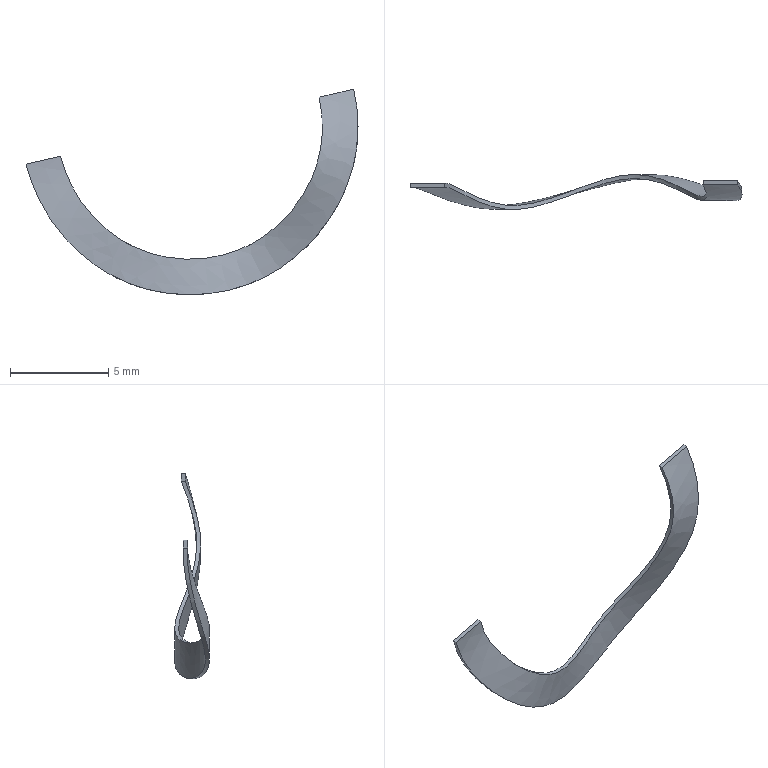Part | NX | features ODD_TURNS_COMBINE 2 | 1 solid | 6 faces | box 16.858 x 1.775 x 10.436 mm | volume 8.764 mm3 | spline 4 | plane 2
STEP:
#1=CARTESIAN_POINT('',(-8.32,-24.173,-1.899));
#2=VERTEX_POINT('',#1);
#3=CARTESIAN_POINT('',(-8.32,-23.97,-1.899));
#4=VERTEX_POINT('',#3);
#5=CARTESIAN_POINT('',(-8.32,-23.97,-1.899));
#6=CARTESIAN_POINT('',(-8.32,-24.037,-1.899));
#7=CARTESIAN_POINT('',(-8.32,-24.105,-1.899));
#8=CARTESIAN_POINT('',(-8.32,-24.173,-1.899));
#9=B_SPLINE_CURVE_WITH_KNOTS('',3,(#5,#6,#7,#8),.UNSPECIFIED.,.F.,.F.,(4,4),(0.,0.0002032),.UNSPECIFIED.);
#10=EDGE_CURVE('',#2,#4,#9,.F.);
#11=ORIENTED_EDGE('',*,*,#10,.T.);
#12=CARTESIAN_POINT('',(8.322,-23.865,1.899));
#13=VERTEX_POINT('',#12);
#14=CARTESIAN_POINT('',(-3.703,-25.301,-7.689));
#15=CARTESIAN_POINT('',(-1.417,-25.248,-8.753));
#16=CARTESIAN_POINT('',(4.289,-27.759,-8.773));
#17=CARTESIAN_POINT('',(9.501,-23.516,-2.229));
#18=CARTESIAN_POINT('',(7.592,-27.322,6.131));
#19=CARTESIAN_POINT('',(0.06027,-23.071,9.76));
#20=CARTESIAN_POINT('',(-7.667,-26.878,6.037));
#21=CARTESIAN_POINT('',(-9.528,-22.627,-2.113));
#22=CARTESIAN_POINT('',(-4.18,-26.435,-8.819));
#23=CARTESIAN_POINT('',(4.18,-22.183,-8.819));
#24=CARTESIAN_POINT('',(9.527,-25.991,-2.113));
#25=CARTESIAN_POINT('',(7.668,-21.74,6.038));
#26=CARTESIAN_POINT('',(-0.06063,-25.547,9.759));
#27=CARTESIAN_POINT('',(-7.591,-21.298,6.133));
#28=CARTESIAN_POINT('',(-8.865,-23.825,0.5668));
#29=CARTESIAN_POINT('',(-8.32,-23.761,-1.899));
#30=B_SPLINE_CURVE_WITH_KNOTS('',3,(#14,#15,#16,#17,#18,#19,#20,#21,#22,#23,#24,#25,#26,#27,#28,#29),.UNSPECIFIED.,.F.,.F.,(4,1,1,1,1,1,1,1,1,1,1,1,1,4),(0.,0.07646,0.1539,0.2304,0.3078,0.3843,0.4618,0.5382,0.6157,0.6922,0.7696,0.8461,0.9235,1.),.UNSPECIFIED.);
#31=EDGE_CURVE('',#4,#13,#30,.T.);
#32=ORIENTED_EDGE('',*,*,#31,.T.);
#33=CARTESIAN_POINT('',(8.322,-24.069,1.899));
#34=VERTEX_POINT('',#33);
#35=CARTESIAN_POINT('',(8.322,-24.069,1.899));
#36=CARTESIAN_POINT('',(8.322,-24.001,1.899));
#37=CARTESIAN_POINT('',(8.322,-23.933,1.899));
#38=CARTESIAN_POINT('',(8.322,-23.865,1.899));
#39=B_SPLINE_CURVE_WITH_KNOTS('',3,(#35,#36,#37,#38),.UNSPECIFIED.,.F.,.F.,(4,4),(0.,0.0002032),.UNSPECIFIED.);
#40=EDGE_CURVE('',#13,#34,#39,.F.);
#41=ORIENTED_EDGE('',*,*,#40,.T.);
#42=CARTESIAN_POINT('',(-3.703,-25.504,-7.689));
#43=CARTESIAN_POINT('',(-1.417,-25.451,-8.753));
#44=CARTESIAN_POINT('',(4.289,-27.962,-8.773));
#45=CARTESIAN_POINT('',(9.501,-23.72,-2.229));
#46=CARTESIAN_POINT('',(7.592,-27.525,6.131));
#47=CARTESIAN_POINT('',(0.06027,-23.274,9.76));
#48=CARTESIAN_POINT('',(-7.667,-27.082,6.037));
#49=CARTESIAN_POINT('',(-9.528,-22.83,-2.113));
#50=CARTESIAN_POINT('',(-4.18,-26.638,-8.819));
#51=CARTESIAN_POINT('',(4.18,-22.387,-8.819));
#52=CARTESIAN_POINT('',(9.527,-26.194,-2.113));
#53=CARTESIAN_POINT('',(7.668,-21.943,6.038));
#54=CARTESIAN_POINT('',(-0.06063,-25.75,9.759));
#55=CARTESIAN_POINT('',(-7.591,-21.501,6.133));
#56=CARTESIAN_POINT('',(-8.865,-24.028,0.5668));
#57=CARTESIAN_POINT('',(-8.32,-23.964,-1.899));
#58=B_SPLINE_CURVE_WITH_KNOTS('',3,(#42,#43,#44,#45,#46,#47,#48,#49,#50,#51,#52,#53,#54,#55,#56,#57),.UNSPECIFIED.,.F.,.F.,(4,1,1,1,1,1,1,1,1,1,1,1,1,4),(0.,0.07646,0.1539,0.2304,0.3078,0.3843,0.4618,0.5382,0.6157,0.6922,0.7696,0.8461,0.9235,1.),.UNSPECIFIED.);
#59=EDGE_CURVE('',#2,#34,#58,.T.);
#60=ORIENTED_EDGE('',*,*,#59,.F.);
#61=EDGE_LOOP('',(#11,#32,#41,#60));
#62=FACE_BOUND('',#61,.T.);
#63=CARTESIAN_POINT('',(-8.32,-24.173,-1.899));
#64=CARTESIAN_POINT('',(-7.737,-24.105,-4.358));
#65=CARTESIAN_POINT('',(-4.18,-26.638,-8.819));
#66=CARTESIAN_POINT('',(4.18,-22.387,-8.819));
#67=CARTESIAN_POINT('',(8.632,-25.557,-3.235));
#68=CARTESIAN_POINT('',(8.606,-24.443,0.6545));
#69=CARTESIAN_POINT('',(8.322,-24.069,1.899));
#70=CARTESIAN_POINT('',(-8.32,-24.156,-1.899));
#71=CARTESIAN_POINT('',(-7.737,-24.088,-4.358));
#72=CARTESIAN_POINT('',(-4.18,-26.621,-8.819));
#73=CARTESIAN_POINT('',(4.18,-22.37,-8.819));
#74=CARTESIAN_POINT('',(8.632,-25.54,-3.235));
#75=CARTESIAN_POINT('',(8.606,-24.426,0.6545));
#76=CARTESIAN_POINT('',(8.322,-24.052,1.899));
#77=CARTESIAN_POINT('',(-8.32,-24.122,-1.899));
#78=CARTESIAN_POINT('',(-7.737,-24.054,-4.358));
#79=CARTESIAN_POINT('',(-4.18,-26.587,-8.819));
#80=CARTESIAN_POINT('',(4.18,-22.336,-8.819));
#81=CARTESIAN_POINT('',(8.632,-25.506,-3.235));
#82=CARTESIAN_POINT('',(8.606,-24.392,0.6545));
#83=CARTESIAN_POINT('',(8.322,-24.018,1.899));
#84=CARTESIAN_POINT('',(-8.32,-24.071,-1.899));
#85=CARTESIAN_POINT('',(-7.737,-24.003,-4.358));
#86=CARTESIAN_POINT('',(-4.18,-26.536,-8.819));
#87=CARTESIAN_POINT('',(4.18,-22.285,-8.819));
#88=CARTESIAN_POINT('',(8.632,-25.455,-3.235));
#89=CARTESIAN_POINT('',(8.606,-24.342,0.6545));
#90=CARTESIAN_POINT('',(8.322,-23.967,1.899));
#91=CARTESIAN_POINT('',(-8.32,-24.02,-1.899));
#92=CARTESIAN_POINT('',(-7.737,-23.953,-4.358));
#93=CARTESIAN_POINT('',(-4.18,-26.486,-8.819));
#94=CARTESIAN_POINT('',(4.18,-22.234,-8.819));
#95=CARTESIAN_POINT('',(8.632,-25.404,-3.235));
#96=CARTESIAN_POINT('',(8.606,-24.291,0.6545));
#97=CARTESIAN_POINT('',(8.322,-23.916,1.899));
#98=CARTESIAN_POINT('',(-8.32,-23.986,-1.899));
#99=CARTESIAN_POINT('',(-7.737,-23.919,-4.358));
#100=CARTESIAN_POINT('',(-4.18,-26.452,-8.819));
#101=CARTESIAN_POINT('',(4.18,-22.2,-8.819));
#102=CARTESIAN_POINT('',(8.632,-25.371,-3.235));
#103=CARTESIAN_POINT('',(8.606,-24.257,0.6545));
#104=CARTESIAN_POINT('',(8.322,-23.882,1.899));
#105=CARTESIAN_POINT('',(-8.32,-23.97,-1.899));
#106=CARTESIAN_POINT('',(-7.737,-23.902,-4.358));
#107=CARTESIAN_POINT('',(-4.18,-26.435,-8.819));
#108=CARTESIAN_POINT('',(4.18,-22.183,-8.819));
#109=CARTESIAN_POINT('',(8.632,-25.354,-3.235));
#110=CARTESIAN_POINT('',(8.606,-24.24,0.6545));
#111=CARTESIAN_POINT('',(8.322,-23.865,1.899));
#112=B_SPLINE_SURFACE_WITH_KNOTS('',3,3,((#63,#64,#65,#66,#67,#68,#69),(#70,#71,#72,#73,#74,#75,#76),(#77,#78,#79,#80,#81,#82,#83),(#84,#85,#86,#87,#88,#89,#90),(#91,#92,#93,#94,#95,#96,#97),(#98,#99,#100,#101,#102,#103,#104),(#105,#106,#107,#108,#109,#110,#111)),.SURF_OF_LINEAR_EXTRUSION.,.F.,.F.,.F.,(4,1,1,1,4),(4,1,1,1,4),(0.,0.25,0.5,0.75,1.),(0.4503,0.5,0.5503,0.6,0.6252),.UNSPECIFIED.);
#113=ADVANCED_FACE('',(#62),#112,.T.);
#114=CARTESIAN_POINT('',(-6.562,-24.173,-1.498));
#115=VERTEX_POINT('',#114);
#116=CARTESIAN_POINT('',(-8.32,-24.173,-1.899));
#117=CARTESIAN_POINT('',(-7.734,-24.173,-1.765));
#118=CARTESIAN_POINT('',(-7.148,-24.173,-1.631));
#119=CARTESIAN_POINT('',(-6.562,-24.173,-1.498));
#120=B_SPLINE_CURVE_WITH_KNOTS('',3,(#116,#117,#118,#119),.UNSPECIFIED.,.F.,.F.,(4,4),(0.,0.001803),.UNSPECIFIED.);
#121=EDGE_CURVE('',#2,#115,#120,.T.);
#122=ORIENTED_EDGE('',*,*,#121,.F.);
#123=ORIENTED_EDGE('',*,*,#59,.T.);
#124=CARTESIAN_POINT('',(6.564,-24.069,1.498));
#125=VERTEX_POINT('',#124);
#126=CARTESIAN_POINT('',(6.564,-24.069,1.498));
#127=CARTESIAN_POINT('',(7.15,-24.069,1.632));
#128=CARTESIAN_POINT('',(7.736,-24.069,1.766));
#129=CARTESIAN_POINT('',(8.322,-24.069,1.899));
#130=B_SPLINE_CURVE_WITH_KNOTS('',3,(#126,#127,#128,#129),.UNSPECIFIED.,.F.,.F.,(4,4),(0.,0.001804),.UNSPECIFIED.);
#131=EDGE_CURVE('',#125,#34,#130,.T.);
#132=ORIENTED_EDGE('',*,*,#131,.F.);
#133=CARTESIAN_POINT('',(-2.92,-25.504,-6.064));
#134=CARTESIAN_POINT('',(-1.118,-25.451,-6.904));
#135=CARTESIAN_POINT('',(3.383,-27.962,-6.919));
#136=CARTESIAN_POINT('',(7.493,-23.72,-1.758));
#137=CARTESIAN_POINT('',(5.988,-27.525,4.836));
#138=CARTESIAN_POINT('',(0.04752,-23.274,7.697));
#139=CARTESIAN_POINT('',(-6.047,-27.082,4.761));
#140=CARTESIAN_POINT('',(-7.514,-22.83,-1.666));
#141=CARTESIAN_POINT('',(-3.297,-26.638,-6.955));
#142=CARTESIAN_POINT('',(3.297,-22.387,-6.955));
#143=CARTESIAN_POINT('',(7.514,-26.194,-1.666));
#144=CARTESIAN_POINT('',(6.047,-21.943,4.762));
#145=CARTESIAN_POINT('',(-0.04783,-25.75,7.697));
#146=CARTESIAN_POINT('',(-5.987,-21.501,4.837));
#147=CARTESIAN_POINT('',(-6.991,-24.028,0.447));
#148=CARTESIAN_POINT('',(-6.562,-23.964,-1.498));
#149=B_SPLINE_CURVE_WITH_KNOTS('',3,(#133,#134,#135,#136,#137,#138,#139,#140,#141,#142,#143,#144,#145,#146,#147,#148),.UNSPECIFIED.,.F.,.F.,(4,1,1,1,1,1,1,1,1,1,1,1,1,4),(0.,0.07646,0.1539,0.2304,0.3078,0.3843,0.4618,0.5382,0.6157,0.6922,0.7696,0.8461,0.9235,1.),.UNSPECIFIED.);
#150=EDGE_CURVE('',#115,#125,#149,.T.);
#151=ORIENTED_EDGE('',*,*,#150,.F.);
#152=EDGE_LOOP('',(#122,#123,#132,#151));
#153=FACE_BOUND('',#152,.T.);
#154=CARTESIAN_POINT('',(-6.562,-24.173,-1.498));
#155=CARTESIAN_POINT('',(-6.102,-24.105,-3.437));
#156=CARTESIAN_POINT('',(-3.297,-26.638,-6.955));
#157=CARTESIAN_POINT('',(3.297,-22.387,-6.955));
#158=CARTESIAN_POINT('',(6.838,-25.583,-2.515));
#159=CARTESIAN_POINT('',(6.787,-24.411,0.6023));
#160=CARTESIAN_POINT('',(6.534,-24.022,1.621));
#161=CARTESIAN_POINT('',(-6.708,-24.173,-1.531));
#162=CARTESIAN_POINT('',(-6.239,-24.105,-3.514));
#163=CARTESIAN_POINT('',(-3.37,-26.638,-7.111));
#164=CARTESIAN_POINT('',(3.37,-22.387,-7.111));
#165=CARTESIAN_POINT('',(6.99,-25.583,-2.571));
#166=CARTESIAN_POINT('',(6.938,-24.411,0.6157));
#167=CARTESIAN_POINT('',(6.68,-24.022,1.657));
#168=CARTESIAN_POINT('',(-7.001,-24.173,-1.598));
#169=CARTESIAN_POINT('',(-6.511,-24.105,-3.667));
#170=CARTESIAN_POINT('',(-3.518,-26.638,-7.421));
#171=CARTESIAN_POINT('',(3.518,-22.387,-7.421));
#172=CARTESIAN_POINT('',(7.296,-25.583,-2.683));
#173=CARTESIAN_POINT('',(7.241,-24.411,0.6426));
#174=CARTESIAN_POINT('',(6.972,-24.022,1.729));
#175=CARTESIAN_POINT('',(-7.441,-24.173,-1.698));
#176=CARTESIAN_POINT('',(-6.92,-24.105,-3.897));
#177=CARTESIAN_POINT('',(-3.739,-26.638,-7.887));
#178=CARTESIAN_POINT('',(3.739,-22.387,-7.887));
#179=CARTESIAN_POINT('',(7.754,-25.583,-2.852));
#180=CARTESIAN_POINT('',(7.696,-24.411,0.6829));
#181=CARTESIAN_POINT('',(7.41,-24.022,1.838));
#182=CARTESIAN_POINT('',(-7.88,-24.173,-1.799));
#183=CARTESIAN_POINT('',(-7.329,-24.105,-4.128));
#184=CARTESIAN_POINT('',(-3.959,-26.638,-8.353));
#185=CARTESIAN_POINT('',(3.959,-22.387,-8.353));
#186=CARTESIAN_POINT('',(8.212,-25.583,-3.02));
#187=CARTESIAN_POINT('',(8.15,-24.411,0.7233));
#188=CARTESIAN_POINT('',(7.848,-24.022,1.946));
#189=CARTESIAN_POINT('',(-8.173,-24.173,-1.866));
#190=CARTESIAN_POINT('',(-7.601,-24.105,-4.281));
#191=CARTESIAN_POINT('',(-4.107,-26.638,-8.664));
#192=CARTESIAN_POINT('',(4.107,-22.387,-8.664));
#193=CARTESIAN_POINT('',(8.517,-25.583,-3.132));
#194=CARTESIAN_POINT('',(8.454,-24.411,0.7502));
#195=CARTESIAN_POINT('',(8.139,-24.022,2.019));
#196=CARTESIAN_POINT('',(-8.32,-24.173,-1.899));
#197=CARTESIAN_POINT('',(-7.737,-24.105,-4.358));
#198=CARTESIAN_POINT('',(-4.18,-26.638,-8.819));
#199=CARTESIAN_POINT('',(4.18,-22.387,-8.819));
#200=CARTESIAN_POINT('',(8.67,-25.583,-3.189));
#201=CARTESIAN_POINT('',(8.605,-24.411,0.7636));
#202=CARTESIAN_POINT('',(8.285,-24.022,2.055));
#203=B_SPLINE_SURFACE_WITH_KNOTS('',3,3,((#154,#155,#156,#157,#158,#159,#160),(#161,#162,#163,#164,#165,#166,#167),(#168,#169,#170,#171,#172,#173,#174),(#175,#176,#177,#178,#179,#180,#181),(#182,#183,#184,#185,#186,#187,#188),(#189,#190,#191,#192,#193,#194,#195),(#196,#197,#198,#199,#200,#201,#202)),.RULED_SURF.,.F.,.F.,.F.,(4,1,1,1,4),(4,1,1,1,4),(0.,0.25,0.5,0.75,1.),(0.4503,0.5,0.5503,0.6,0.6262),.UNSPECIFIED.);
#204=ADVANCED_FACE('',(#153),#203,.T.);
#205=CARTESIAN_POINT('',(-6.562,-23.97,-1.498));
#206=VERTEX_POINT('',#205);
#207=CARTESIAN_POINT('',(-6.562,-23.97,-1.498));
#208=CARTESIAN_POINT('',(-7.148,-23.97,-1.631));
#209=CARTESIAN_POINT('',(-7.734,-23.97,-1.765));
#210=CARTESIAN_POINT('',(-8.32,-23.97,-1.899));
#211=B_SPLINE_CURVE_WITH_KNOTS('',3,(#207,#208,#209,#210),.UNSPECIFIED.,.F.,.F.,(4,4),(0.,0.001803),.UNSPECIFIED.);
#212=EDGE_CURVE('',#206,#4,#211,.T.);
#213=ORIENTED_EDGE('',*,*,#212,.F.);
#214=CARTESIAN_POINT('',(6.564,-23.865,1.498));
#215=VERTEX_POINT('',#214);
#216=CARTESIAN_POINT('',(-2.92,-25.301,-6.064));
#217=CARTESIAN_POINT('',(-1.118,-25.248,-6.904));
#218=CARTESIAN_POINT('',(3.383,-27.759,-6.919));
#219=CARTESIAN_POINT('',(7.493,-23.516,-1.758));
#220=CARTESIAN_POINT('',(5.988,-27.322,4.836));
#221=CARTESIAN_POINT('',(0.04752,-23.071,7.697));
#222=CARTESIAN_POINT('',(-6.047,-26.878,4.761));
#223=CARTESIAN_POINT('',(-7.514,-22.627,-1.666));
#224=CARTESIAN_POINT('',(-3.297,-26.435,-6.955));
#225=CARTESIAN_POINT('',(3.297,-22.183,-6.955));
#226=CARTESIAN_POINT('',(7.514,-25.991,-1.666));
#227=CARTESIAN_POINT('',(6.047,-21.74,4.762));
#228=CARTESIAN_POINT('',(-0.04783,-25.547,7.697));
#229=CARTESIAN_POINT('',(-5.987,-21.298,4.837));
#230=CARTESIAN_POINT('',(-6.991,-23.825,0.447));
#231=CARTESIAN_POINT('',(-6.562,-23.761,-1.498));
#232=B_SPLINE_CURVE_WITH_KNOTS('',3,(#216,#217,#218,#219,#220,#221,#222,#223,#224,#225,#226,#227,#228,#229,#230,#231),.UNSPECIFIED.,.F.,.F.,(4,1,1,1,1,1,1,1,1,1,1,1,1,4),(0.,0.07646,0.1539,0.2304,0.3078,0.3843,0.4618,0.5382,0.6157,0.6922,0.7696,0.8461,0.9235,1.),.UNSPECIFIED.);
#233=EDGE_CURVE('',#206,#215,#232,.T.);
#234=ORIENTED_EDGE('',*,*,#233,.T.);
#235=CARTESIAN_POINT('',(8.322,-23.865,1.899));
#236=CARTESIAN_POINT('',(7.736,-23.865,1.766));
#237=CARTESIAN_POINT('',(7.15,-23.865,1.632));
#238=CARTESIAN_POINT('',(6.564,-23.865,1.498));
#239=B_SPLINE_CURVE_WITH_KNOTS('',3,(#235,#236,#237,#238),.UNSPECIFIED.,.F.,.F.,(4,4),(0.,0.001804),.UNSPECIFIED.);
#240=EDGE_CURVE('',#13,#215,#239,.T.);
#241=ORIENTED_EDGE('',*,*,#240,.F.);
#242=ORIENTED_EDGE('',*,*,#31,.F.);
#243=EDGE_LOOP('',(#213,#234,#241,#242));
#244=FACE_BOUND('',#243,.T.);
#245=CARTESIAN_POINT('',(-8.32,-23.97,-1.899));
#246=CARTESIAN_POINT('',(-7.737,-23.902,-4.358));
#247=CARTESIAN_POINT('',(-4.18,-26.435,-8.819));
#248=CARTESIAN_POINT('',(4.18,-22.183,-8.819));
#249=CARTESIAN_POINT('',(8.67,-25.38,-3.189));
#250=CARTESIAN_POINT('',(8.605,-24.208,0.7636));
#251=CARTESIAN_POINT('',(8.285,-23.819,2.055));
#252=CARTESIAN_POINT('',(-8.247,-23.97,-1.882));
#253=CARTESIAN_POINT('',(-7.669,-23.902,-4.319));
#254=CARTESIAN_POINT('',(-4.143,-26.435,-8.741));
#255=CARTESIAN_POINT('',(4.143,-22.183,-8.741));
#256=CARTESIAN_POINT('',(8.593,-25.38,-3.16));
#257=CARTESIAN_POINT('',(8.529,-24.208,0.7569));
#258=CARTESIAN_POINT('',(8.212,-23.819,2.037));
#259=CARTESIAN_POINT('',(-8.1,-23.97,-1.849));
#260=CARTESIAN_POINT('',(-7.533,-23.902,-4.243));
#261=CARTESIAN_POINT('',(-4.07,-26.435,-8.586));
#262=CARTESIAN_POINT('',(4.07,-22.183,-8.586));
#263=CARTESIAN_POINT('',(8.441,-25.38,-3.104));
#264=CARTESIAN_POINT('',(8.378,-24.208,0.7434));
#265=CARTESIAN_POINT('',(8.066,-23.819,2.001));
#266=CARTESIAN_POINT('',(-7.88,-23.97,-1.799));
#267=CARTESIAN_POINT('',(-7.329,-23.902,-4.128));
#268=CARTESIAN_POINT('',(-3.959,-26.435,-8.353));
#269=CARTESIAN_POINT('',(3.959,-22.183,-8.353));
#270=CARTESIAN_POINT('',(8.212,-25.38,-3.02));
#271=CARTESIAN_POINT('',(8.15,-24.208,0.7233));
#272=CARTESIAN_POINT('',(7.848,-23.819,1.946));
#273=CARTESIAN_POINT('',(-7.661,-23.97,-1.748));
#274=CARTESIAN_POINT('',(-7.124,-23.902,-4.012));
#275=CARTESIAN_POINT('',(-3.849,-26.435,-8.12));
#276=CARTESIAN_POINT('',(3.849,-22.183,-8.12));
#277=CARTESIAN_POINT('',(7.983,-25.38,-2.936));
#278=CARTESIAN_POINT('',(7.923,-24.208,0.7031));
#279=CARTESIAN_POINT('',(7.629,-23.819,1.892));
#280=CARTESIAN_POINT('',(-7.514,-23.97,-1.715));
#281=CARTESIAN_POINT('',(-6.988,-23.902,-3.936));
#282=CARTESIAN_POINT('',(-3.775,-26.435,-7.965));
#283=CARTESIAN_POINT('',(3.775,-22.183,-7.965));
#284=CARTESIAN_POINT('',(7.83,-25.38,-2.88));
#285=CARTESIAN_POINT('',(7.772,-24.208,0.6897));
#286=CARTESIAN_POINT('',(7.483,-23.819,1.856));
#287=CARTESIAN_POINT('',(-7.368,-23.97,-1.682));
#288=CARTESIAN_POINT('',(-6.852,-23.902,-3.859));
#289=CARTESIAN_POINT('',(-3.702,-26.435,-7.81));
#290=CARTESIAN_POINT('',(3.702,-22.183,-7.81));
#291=CARTESIAN_POINT('',(7.677,-25.38,-2.824));
#292=CARTESIAN_POINT('',(7.62,-24.208,0.6762));
#293=CARTESIAN_POINT('',(7.337,-23.819,1.82));
#294=CARTESIAN_POINT('',(-7.221,-23.97,-1.648));
#295=CARTESIAN_POINT('',(-6.715,-23.902,-3.782));
#296=CARTESIAN_POINT('',(-3.628,-26.435,-7.654));
#297=CARTESIAN_POINT('',(3.628,-22.183,-7.654));
#298=CARTESIAN_POINT('',(7.525,-25.38,-2.767));
#299=CARTESIAN_POINT('',(7.469,-24.208,0.6628));
#300=CARTESIAN_POINT('',(7.191,-23.819,1.783));
#301=CARTESIAN_POINT('',(-7.001,-23.97,-1.598));
#302=CARTESIAN_POINT('',(-6.511,-23.902,-3.667));
#303=CARTESIAN_POINT('',(-3.518,-26.435,-7.421));
#304=CARTESIAN_POINT('',(3.518,-22.183,-7.421));
#305=CARTESIAN_POINT('',(7.296,-25.38,-2.683));
#306=CARTESIAN_POINT('',(7.241,-24.208,0.6426));
#307=CARTESIAN_POINT('',(6.972,-23.819,1.729));
#308=CARTESIAN_POINT('',(-6.782,-23.97,-1.548));
#309=CARTESIAN_POINT('',(-6.307,-23.902,-3.552));
#310=CARTESIAN_POINT('',(-3.407,-26.435,-7.188));
#311=CARTESIAN_POINT('',(3.407,-22.183,-7.188));
#312=CARTESIAN_POINT('',(7.067,-25.38,-2.599));
#313=CARTESIAN_POINT('',(7.014,-24.208,0.6224));
#314=CARTESIAN_POINT('',(6.753,-23.819,1.675));
#315=CARTESIAN_POINT('',(-6.635,-23.97,-1.514));
#316=CARTESIAN_POINT('',(-6.17,-23.902,-3.475));
#317=CARTESIAN_POINT('',(-3.334,-26.435,-7.033));
#318=CARTESIAN_POINT('',(3.334,-22.183,-7.033));
#319=CARTESIAN_POINT('',(6.914,-25.38,-2.543));
#320=CARTESIAN_POINT('',(6.862,-24.208,0.609));
#321=CARTESIAN_POINT('',(6.607,-23.819,1.639));
#322=CARTESIAN_POINT('',(-6.562,-23.97,-1.498));
#323=CARTESIAN_POINT('',(-6.102,-23.902,-3.437));
#324=CARTESIAN_POINT('',(-3.297,-26.435,-6.955));
#325=CARTESIAN_POINT('',(3.297,-22.183,-6.955));
#326=CARTESIAN_POINT('',(6.838,-25.38,-2.515));
#327=CARTESIAN_POINT('',(6.787,-24.208,0.6023));
#328=CARTESIAN_POINT('',(6.534,-23.819,1.621));
#329=B_SPLINE_SURFACE_WITH_KNOTS('',3,3,((#245,#246,#247,#248,#249,#250,#251),(#252,#253,#254,#255,#256,#257,#258),(#259,#260,#261,#262,#263,#264,#265),(#266,#267,#268,#269,#270,#271,#272),(#273,#274,#275,#276,#277,#278,#279),(#280,#281,#282,#283,#284,#285,#286),(#287,#288,#289,#290,#291,#292,#293),(#294,#295,#296,#297,#298,#299,#300),(#301,#302,#303,#304,#305,#306,#307),(#308,#309,#310,#311,#312,#313,#314),(#315,#316,#317,#318,#319,#320,#321),(#322,#323,#324,#325,#326,#327,#328)),.RULED_SURF.,.F.,.F.,.F.,(4,1,1,1,2,1,1,1,4),(4,1,1,1,4),(0.,0.125,0.25,0.375,0.5,0.625,0.75,0.875,1.),(0.4503,0.5,0.5503,0.6,0.6262),.UNSPECIFIED.);
#330=ADVANCED_FACE('',(#244),#329,.T.);
#331=CARTESIAN_POINT('',(-6.562,-24.173,-1.498));
#332=CARTESIAN_POINT('',(-6.562,-24.105,-1.498));
#333=CARTESIAN_POINT('',(-6.562,-24.037,-1.498));
#334=CARTESIAN_POINT('',(-6.562,-23.97,-1.498));
#335=B_SPLINE_CURVE_WITH_KNOTS('',3,(#331,#332,#333,#334),.UNSPECIFIED.,.F.,.F.,(4,4),(0.000001219,0.0002044),.UNSPECIFIED.);
#336=EDGE_CURVE('',#115,#206,#335,.T.);
#337=ORIENTED_EDGE('',*,*,#336,.F.);
#338=ORIENTED_EDGE('',*,*,#150,.T.);
#339=CARTESIAN_POINT('',(6.564,-23.865,1.498));
#340=CARTESIAN_POINT('',(6.564,-23.933,1.498));
#341=CARTESIAN_POINT('',(6.564,-24.001,1.498));
#342=CARTESIAN_POINT('',(6.564,-24.069,1.498));
#343=B_SPLINE_CURVE_WITH_KNOTS('',3,(#339,#340,#341,#342),.UNSPECIFIED.,.F.,.F.,(4,4),(0.,0.0002032),.UNSPECIFIED.);
#344=EDGE_CURVE('',#215,#125,#343,.T.);
#345=ORIENTED_EDGE('',*,*,#344,.F.);
#346=ORIENTED_EDGE('',*,*,#233,.F.);
#347=EDGE_LOOP('',(#337,#338,#345,#346));
#348=FACE_BOUND('',#347,.T.);
#349=CARTESIAN_POINT('',(-6.562,-23.97,-1.498));
#350=CARTESIAN_POINT('',(-6.102,-23.902,-3.437));
#351=CARTESIAN_POINT('',(-3.297,-26.435,-6.955));
#352=CARTESIAN_POINT('',(3.297,-22.183,-6.955));
#353=CARTESIAN_POINT('',(6.808,-25.354,-2.552));
#354=CARTESIAN_POINT('',(6.788,-24.24,0.5162));
#355=CARTESIAN_POINT('',(6.564,-23.865,1.498));
#356=CARTESIAN_POINT('',(-6.562,-23.986,-1.498));
#357=CARTESIAN_POINT('',(-6.102,-23.919,-3.437));
#358=CARTESIAN_POINT('',(-3.297,-26.452,-6.955));
#359=CARTESIAN_POINT('',(3.297,-22.2,-6.955));
#360=CARTESIAN_POINT('',(6.808,-25.371,-2.552));
#361=CARTESIAN_POINT('',(6.788,-24.257,0.5162));
#362=CARTESIAN_POINT('',(6.564,-23.882,1.498));
#363=CARTESIAN_POINT('',(-6.562,-24.02,-1.498));
#364=CARTESIAN_POINT('',(-6.102,-23.953,-3.437));
#365=CARTESIAN_POINT('',(-3.297,-26.486,-6.955));
#366=CARTESIAN_POINT('',(3.297,-22.234,-6.955));
#367=CARTESIAN_POINT('',(6.808,-25.404,-2.552));
#368=CARTESIAN_POINT('',(6.788,-24.291,0.5162));
#369=CARTESIAN_POINT('',(6.564,-23.916,1.498));
#370=CARTESIAN_POINT('',(-6.562,-24.071,-1.498));
#371=CARTESIAN_POINT('',(-6.102,-24.003,-3.437));
#372=CARTESIAN_POINT('',(-3.297,-26.536,-6.955));
#373=CARTESIAN_POINT('',(3.297,-22.285,-6.955));
#374=CARTESIAN_POINT('',(6.808,-25.455,-2.552));
#375=CARTESIAN_POINT('',(6.788,-24.342,0.5162));
#376=CARTESIAN_POINT('',(6.564,-23.967,1.498));
#377=CARTESIAN_POINT('',(-6.562,-24.122,-1.498));
#378=CARTESIAN_POINT('',(-6.102,-24.054,-3.437));
#379=CARTESIAN_POINT('',(-3.297,-26.587,-6.955));
#380=CARTESIAN_POINT('',(3.297,-22.336,-6.955));
#381=CARTESIAN_POINT('',(6.808,-25.506,-2.552));
#382=CARTESIAN_POINT('',(6.788,-24.392,0.5162));
#383=CARTESIAN_POINT('',(6.564,-24.018,1.498));
#384=CARTESIAN_POINT('',(-6.562,-24.156,-1.498));
#385=CARTESIAN_POINT('',(-6.102,-24.088,-3.437));
#386=CARTESIAN_POINT('',(-3.297,-26.621,-6.955));
#387=CARTESIAN_POINT('',(3.297,-22.37,-6.955));
#388=CARTESIAN_POINT('',(6.808,-25.54,-2.552));
#389=CARTESIAN_POINT('',(6.788,-24.426,0.5162));
#390=CARTESIAN_POINT('',(6.564,-24.052,1.498));
#391=CARTESIAN_POINT('',(-6.562,-24.173,-1.498));
#392=CARTESIAN_POINT('',(-6.102,-24.105,-3.437));
#393=CARTESIAN_POINT('',(-3.297,-26.638,-6.955));
#394=CARTESIAN_POINT('',(3.297,-22.387,-6.955));
#395=CARTESIAN_POINT('',(6.808,-25.557,-2.552));
#396=CARTESIAN_POINT('',(6.788,-24.443,0.5162));
#397=CARTESIAN_POINT('',(6.564,-24.069,1.498));
#398=B_SPLINE_SURFACE_WITH_KNOTS('',3,3,((#349,#350,#351,#352,#353,#354,#355),(#356,#357,#358,#359,#360,#361,#362),(#363,#364,#365,#366,#367,#368,#369),(#370,#371,#372,#373,#374,#375,#376),(#377,#378,#379,#380,#381,#382,#383),(#384,#385,#386,#387,#388,#389,#390),(#391,#392,#393,#394,#395,#396,#397)),.SURF_OF_LINEAR_EXTRUSION.,.F.,.F.,.F.,(4,1,1,1,4),(4,1,1,1,4),(0.,0.25,0.5,0.75,1.),(0.4503,0.5,0.5503,0.6,0.6252),.UNSPECIFIED.);
#399=ADVANCED_FACE('',(#348),#398,.T.);
#400=ORIENTED_EDGE('',*,*,#344,.T.);
#401=ORIENTED_EDGE('',*,*,#131,.T.);
#402=ORIENTED_EDGE('',*,*,#40,.F.);
#403=ORIENTED_EDGE('',*,*,#240,.T.);
#404=EDGE_LOOP('',(#400,#401,#402,#403));
#405=FACE_BOUND('',#404,.T.);
#406=CARTESIAN_POINT('',(-8.32,-23.761,-1.899));
#407=DIRECTION('',(0.2225,0.,-0.9749));
#408=DIRECTION('',(-0.9749,0.,-0.2225));
#409=AXIS2_PLACEMENT_3D('',#406,#407,#408);
#410=PLANE('',#409);
#411=ADVANCED_FACE('',(#405),#410,.F.);
#412=ORIENTED_EDGE('',*,*,#336,.T.);
#413=ORIENTED_EDGE('',*,*,#212,.T.);
#414=ORIENTED_EDGE('',*,*,#10,.F.);
#415=ORIENTED_EDGE('',*,*,#121,.T.);
#416=EDGE_LOOP('',(#412,#413,#414,#415));
#417=FACE_BOUND('',#416,.T.);
#418=CARTESIAN_POINT('',(-8.32,-23.761,-1.899));
#419=DIRECTION('',(0.2225,0.,-0.9749));
#420=DIRECTION('',(-0.9749,0.,-0.2225));
#421=AXIS2_PLACEMENT_3D('',#418,#419,#420);
#422=PLANE('',#421);
#423=ADVANCED_FACE('',(#417),#422,.F.);
#424=CLOSED_SHELL('',(#113,#204,#330,#399,#411,#423));
#425=MANIFOLD_SOLID_BREP('',#424);
#426=(LENGTH_UNIT()NAMED_UNIT(*)SI_UNIT(.MILLI.,.METRE.));
#427=UNCERTAINTY_MEASURE_WITH_UNIT(LENGTH_MEASURE(0.0508),#426,'','');
#428=(NAMED_UNIT(*)PLANE_ANGLE_UNIT()SI_UNIT($,.RADIAN.));
#429=(NAMED_UNIT(*)SI_UNIT($,.STERADIAN.)SOLID_ANGLE_UNIT());
#430=(GEOMETRIC_REPRESENTATION_CONTEXT(3)GLOBAL_UNCERTAINTY_ASSIGNED_CONTEXT((#427))GLOBAL_UNIT_ASSIGNED_CONTEXT((#426,#428,#429))REPRESENTATION_CONTEXT('',''));
#431=ADVANCED_BREP_SHAPE_REPRESENTATION('',(#425),#430);